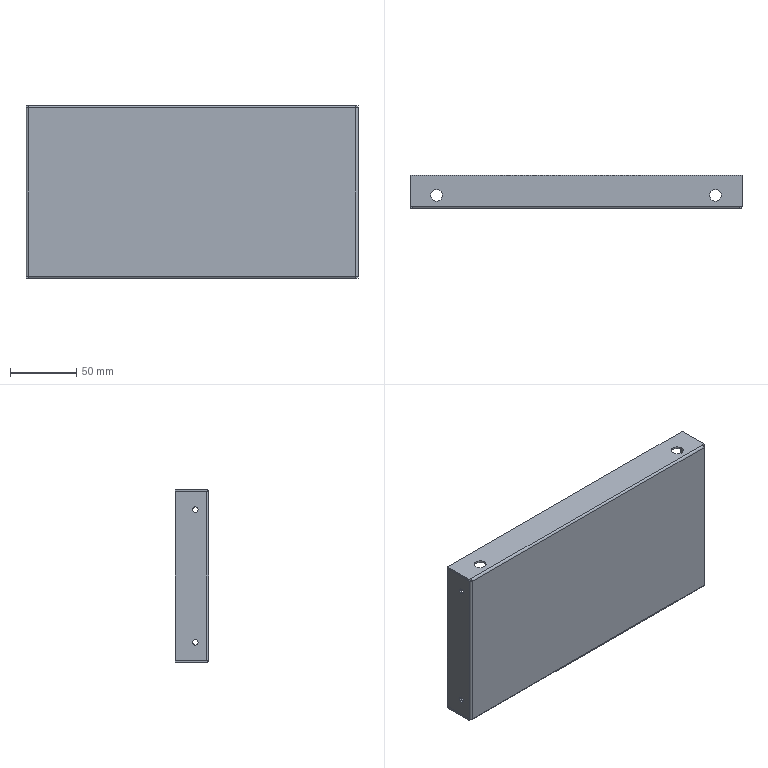Part | STEP file | 1 solid | 58 faces | box 250 x 25 x 130 mm | volume 74457 mm3 | plane 34 | cylinder 24 | commonest cylinder face diameters 4.2 x8 9 x8 0.1 x4 3.1 x4